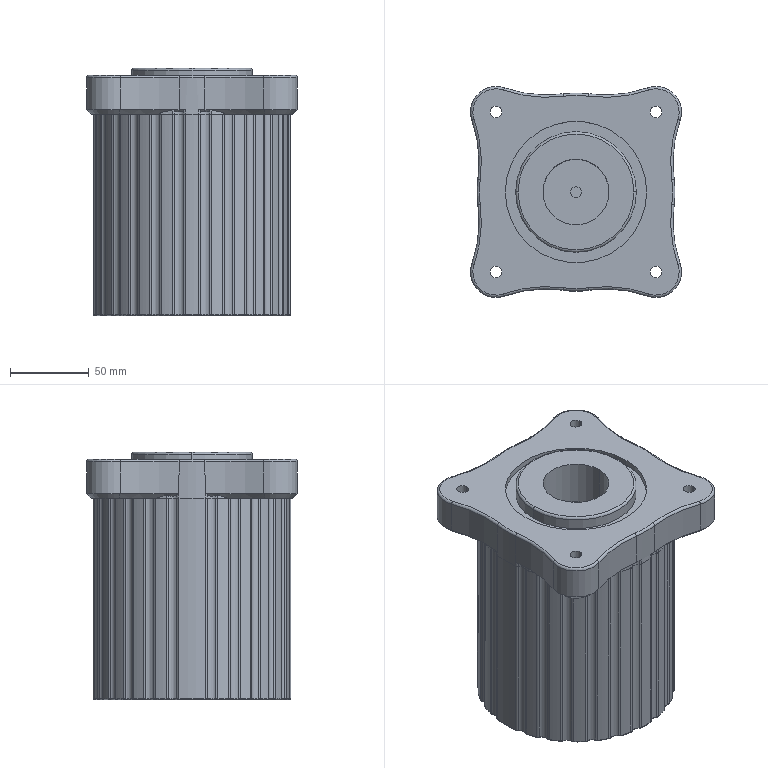Part | SolidWorks | features BaseBody 2 | 2 solids | 354 faces | box 134.4 x 134.4 x 157.5 mm | volume 1797413 mm3 | cylinder 189 | torus 123 | plane 24 | cone 16 | spline 2 | commonest cylinder face diameters 4.2 x68 9 x36 126 x36 1.2 x10 7.5 x8 162 x8